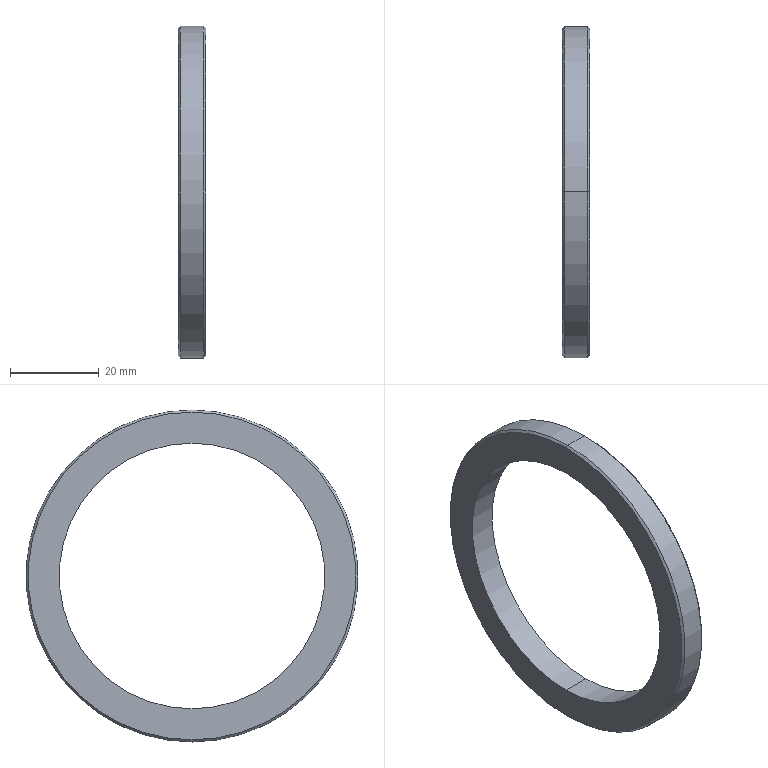Part | SolidWorks | features MBimport 1 | 1 solid | 10 faces | box 6.3 x 75 x 75 mm | volume 9961 mm3 | cone 4 | cylinder 4 | plane 2 | commonest cylinder face diameters 60 x2 75 x2
STEP:
#1=CARTESIAN_POINT('',(-37.414,0.,37.));
#2=VERTEX_POINT('',#1);
#3=CARTESIAN_POINT('',(-36.914,0.,37.5));
#4=VERTEX_POINT('',#3);
#5=CARTESIAN_POINT('',(-36.914,0.,37.5));
#6=DIRECTION('',(0.7071,0.,0.7071));
#7=VECTOR('',#6,1000.);
#8=LINE('',#5,#7);
#9=EDGE_CURVE('',#2,#4,#8,.T.);
#10=ORIENTED_EDGE('',*,*,#9,.F.);
#11=CARTESIAN_POINT('',(-37.414,0.,-37.));
#12=VERTEX_POINT('',#11);
#13=CARTESIAN_POINT('',(-37.414,0.,0.));
#14=DIRECTION('',(-1.,0.,0.));
#15=DIRECTION('',(0.,0.,1.));
#16=AXIS2_PLACEMENT_3D('',#13,#14,#15);
#17=CIRCLE('',#16,37.);
#18=EDGE_CURVE('',#12,#2,#17,.T.);
#19=ORIENTED_EDGE('',*,*,#18,.F.);
#20=CARTESIAN_POINT('',(-36.914,0.,-37.5));
#21=VERTEX_POINT('',#20);
#22=CARTESIAN_POINT('',(-36.914,0.,-37.5));
#23=DIRECTION('',(0.7071,0.,-0.7071));
#24=VECTOR('',#23,1000.);
#25=LINE('',#22,#24);
#26=EDGE_CURVE('',#12,#21,#25,.T.);
#27=ORIENTED_EDGE('',*,*,#26,.T.);
#28=CARTESIAN_POINT('',(-36.914,0.,0.));
#29=DIRECTION('',(1.,0.,0.));
#30=DIRECTION('',(0.,0.,1.));
#31=AXIS2_PLACEMENT_3D('',#28,#29,#30);
#32=CIRCLE('',#31,37.5);
#33=EDGE_CURVE('',#4,#21,#32,.T.);
#34=ORIENTED_EDGE('',*,*,#33,.F.);
#35=EDGE_LOOP('',(#10,#19,#27,#34));
#36=FACE_OUTER_BOUND('',#35,.T.);
#37=CARTESIAN_POINT('',(-36.914,0.,0.));
#38=DIRECTION('',(1.,0.,0.));
#39=DIRECTION('',(0.,0.,-1.));
#40=AXIS2_PLACEMENT_3D('',#37,#38,#39);
#41=CONICAL_SURFACE('',#40,37.5,0.7854);
#42=ADVANCED_FACE('',(#36),#41,.T.);
#43=CARTESIAN_POINT('',(-31.114,0.,-37.));
#44=VERTEX_POINT('',#43);
#45=CARTESIAN_POINT('',(-31.614,0.,-37.5));
#46=VERTEX_POINT('',#45);
#47=CARTESIAN_POINT('',(-31.114,0.,-37.));
#48=DIRECTION('',(-0.7071,0.,-0.7071));
#49=VECTOR('',#48,1000.);
#50=LINE('',#47,#49);
#51=EDGE_CURVE('',#44,#46,#50,.T.);
#52=ORIENTED_EDGE('',*,*,#51,.F.);
#53=CARTESIAN_POINT('',(-31.114,0.,37.));
#54=VERTEX_POINT('',#53);
#55=CARTESIAN_POINT('',(-31.114,0.,0.));
#56=DIRECTION('',(1.,0.,0.));
#57=DIRECTION('',(0.,0.,-1.));
#58=AXIS2_PLACEMENT_3D('',#55,#56,#57);
#59=CIRCLE('',#58,37.);
#60=EDGE_CURVE('',#54,#44,#59,.T.);
#61=ORIENTED_EDGE('',*,*,#60,.F.);
#62=CARTESIAN_POINT('',(-31.614,0.,37.5));
#63=VERTEX_POINT('',#62);
#64=CARTESIAN_POINT('',(-31.114,0.,37.));
#65=DIRECTION('',(-0.7071,0.,0.7071));
#66=VECTOR('',#65,1000.);
#67=LINE('',#64,#66);
#68=EDGE_CURVE('',#54,#63,#67,.T.);
#69=ORIENTED_EDGE('',*,*,#68,.T.);
#70=CARTESIAN_POINT('',(-31.614,0.,0.));
#71=DIRECTION('',(-1.,0.,0.));
#72=DIRECTION('',(0.,0.,-1.));
#73=AXIS2_PLACEMENT_3D('',#70,#71,#72);
#74=CIRCLE('',#73,37.5);
#75=EDGE_CURVE('',#46,#63,#74,.T.);
#76=ORIENTED_EDGE('',*,*,#75,.F.);
#77=EDGE_LOOP('',(#52,#61,#69,#76));
#78=FACE_OUTER_BOUND('',#77,.T.);
#79=CARTESIAN_POINT('',(-31.114,0.,0.));
#80=DIRECTION('',(-1.,0.,0.));
#81=DIRECTION('',(0.,0.,1.));
#82=AXIS2_PLACEMENT_3D('',#79,#80,#81);
#83=CONICAL_SURFACE('',#82,37.,0.7854);
#84=ADVANCED_FACE('',(#78),#83,.T.);
#85=CARTESIAN_POINT('',(0.,0.,37.5));
#86=DIRECTION('',(1.,0.,0.));
#87=VECTOR('',#86,1000.);
#88=LINE('',#85,#87);
#89=EDGE_CURVE('',#4,#63,#88,.T.);
#90=ORIENTED_EDGE('',*,*,#89,.F.);
#91=ORIENTED_EDGE('',*,*,#33,.T.);
#92=CARTESIAN_POINT('',(0.,0.,-37.5));
#93=DIRECTION('',(1.,0.,0.));
#94=VECTOR('',#93,1000.);
#95=LINE('',#92,#94);
#96=EDGE_CURVE('',#21,#46,#95,.T.);
#97=ORIENTED_EDGE('',*,*,#96,.T.);
#98=ORIENTED_EDGE('',*,*,#75,.T.);
#99=EDGE_LOOP('',(#90,#91,#97,#98));
#100=FACE_OUTER_BOUND('',#99,.T.);
#101=CARTESIAN_POINT('',(0.,0.,0.));
#102=DIRECTION('',(1.,0.,0.));
#103=DIRECTION('',(0.,0.,-1.));
#104=AXIS2_PLACEMENT_3D('',#101,#102,#103);
#105=CYLINDRICAL_SURFACE('',#104,37.5);
#106=ADVANCED_FACE('',(#100),#105,.T.);
#107=CARTESIAN_POINT('',(-31.114,0.,-30.));
#108=VERTEX_POINT('',#107);
#109=CARTESIAN_POINT('',(-31.114,0.,30.));
#110=VERTEX_POINT('',#109);
#111=CARTESIAN_POINT('',(-31.114,0.,0.));
#112=DIRECTION('',(1.,0.,0.));
#113=DIRECTION('',(0.,0.,-1.));
#114=AXIS2_PLACEMENT_3D('',#111,#112,#113);
#115=CIRCLE('',#114,30.);
#116=EDGE_CURVE('',#108,#110,#115,.T.);
#117=ORIENTED_EDGE('',*,*,#116,.F.);
#118=CARTESIAN_POINT('',(-31.114,0.,0.));
#119=DIRECTION('',(1.,0.,0.));
#120=DIRECTION('',(0.,0.,-1.));
#121=AXIS2_PLACEMENT_3D('',#118,#119,#120);
#122=CIRCLE('',#121,30.);
#123=EDGE_CURVE('',#110,#108,#122,.T.);
#124=ORIENTED_EDGE('',*,*,#123,.F.);
#125=EDGE_LOOP('',(#117,#124));
#126=FACE_BOUND('',#125,.T.);
#127=ORIENTED_EDGE('',*,*,#60,.T.);
#128=CARTESIAN_POINT('',(-31.114,0.,0.));
#129=DIRECTION('',(1.,0.,0.));
#130=DIRECTION('',(0.,0.,-1.));
#131=AXIS2_PLACEMENT_3D('',#128,#129,#130);
#132=CIRCLE('',#131,37.);
#133=EDGE_CURVE('',#44,#54,#132,.T.);
#134=ORIENTED_EDGE('',*,*,#133,.T.);
#135=EDGE_LOOP('',(#127,#134));
#136=FACE_OUTER_BOUND('',#135,.T.);
#137=CARTESIAN_POINT('',(-31.114,37.5,0.));
#138=DIRECTION('',(1.,0.,0.));
#139=DIRECTION('',(0.,1.,0.));
#140=AXIS2_PLACEMENT_3D('',#137,#138,#139);
#141=PLANE('',#140);
#142=ADVANCED_FACE('',(#126,#136),#141,.T.);
#143=CARTESIAN_POINT('',(-37.414,0.,30.));
#144=VERTEX_POINT('',#143);
#145=CARTESIAN_POINT('',(0.,0.,30.));
#146=DIRECTION('',(1.,0.,0.));
#147=VECTOR('',#146,1000.);
#148=LINE('',#145,#147);
#149=EDGE_CURVE('',#144,#110,#148,.T.);
#150=ORIENTED_EDGE('',*,*,#149,.F.);
#151=CARTESIAN_POINT('',(-37.414,0.,-30.));
#152=VERTEX_POINT('',#151);
#153=CARTESIAN_POINT('',(-37.414,0.,0.));
#154=DIRECTION('',(1.,0.,0.));
#155=DIRECTION('',(0.,0.,-1.));
#156=AXIS2_PLACEMENT_3D('',#153,#154,#155);
#157=CIRCLE('',#156,30.);
#158=EDGE_CURVE('',#152,#144,#157,.T.);
#159=ORIENTED_EDGE('',*,*,#158,.F.);
#160=CARTESIAN_POINT('',(0.,0.,-30.));
#161=DIRECTION('',(1.,0.,0.));
#162=VECTOR('',#161,1000.);
#163=LINE('',#160,#162);
#164=EDGE_CURVE('',#152,#108,#163,.T.);
#165=ORIENTED_EDGE('',*,*,#164,.T.);
#166=ORIENTED_EDGE('',*,*,#116,.T.);
#167=EDGE_LOOP('',(#150,#159,#165,#166));
#168=FACE_OUTER_BOUND('',#167,.T.);
#169=CARTESIAN_POINT('',(0.,0.,0.));
#170=DIRECTION('',(1.,0.,0.));
#171=DIRECTION('',(0.,0.,-1.));
#172=AXIS2_PLACEMENT_3D('',#169,#170,#171);
#173=CYLINDRICAL_SURFACE('',#172,30.);
#174=ADVANCED_FACE('',(#168),#173,.F.);
#175=ORIENTED_EDGE('',*,*,#158,.T.);
#176=CARTESIAN_POINT('',(-37.414,0.,0.));
#177=DIRECTION('',(1.,0.,0.));
#178=DIRECTION('',(0.,0.,-1.));
#179=AXIS2_PLACEMENT_3D('',#176,#177,#178);
#180=CIRCLE('',#179,30.);
#181=EDGE_CURVE('',#144,#152,#180,.T.);
#182=ORIENTED_EDGE('',*,*,#181,.T.);
#183=EDGE_LOOP('',(#175,#182));
#184=FACE_BOUND('',#183,.T.);
#185=ORIENTED_EDGE('',*,*,#18,.T.);
#186=CARTESIAN_POINT('',(-37.414,0.,0.));
#187=DIRECTION('',(-1.,0.,0.));
#188=DIRECTION('',(0.,0.,1.));
#189=AXIS2_PLACEMENT_3D('',#186,#187,#188);
#190=CIRCLE('',#189,37.);
#191=EDGE_CURVE('',#2,#12,#190,.T.);
#192=ORIENTED_EDGE('',*,*,#191,.T.);
#193=EDGE_LOOP('',(#185,#192));
#194=FACE_OUTER_BOUND('',#193,.T.);
#195=CARTESIAN_POINT('',(-37.414,37.5,0.));
#196=DIRECTION('',(-1.,0.,0.));
#197=DIRECTION('',(0.,0.,1.));
#198=AXIS2_PLACEMENT_3D('',#195,#196,#197);
#199=PLANE('',#198);
#200=ADVANCED_FACE('',(#184,#194),#199,.T.);
#201=ORIENTED_EDGE('',*,*,#181,.F.);
#202=ORIENTED_EDGE('',*,*,#149,.T.);
#203=ORIENTED_EDGE('',*,*,#123,.T.);
#204=ORIENTED_EDGE('',*,*,#164,.F.);
#205=EDGE_LOOP('',(#201,#202,#203,#204));
#206=FACE_OUTER_BOUND('',#205,.T.);
#207=CARTESIAN_POINT('',(0.,0.,0.));
#208=DIRECTION('',(1.,0.,0.));
#209=DIRECTION('',(0.,0.,-1.));
#210=AXIS2_PLACEMENT_3D('',#207,#208,#209);
#211=CYLINDRICAL_SURFACE('',#210,30.);
#212=ADVANCED_FACE('',(#206),#211,.F.);
#213=CARTESIAN_POINT('',(-36.914,0.,0.));
#214=DIRECTION('',(1.,0.,0.));
#215=DIRECTION('',(0.,0.,1.));
#216=AXIS2_PLACEMENT_3D('',#213,#214,#215);
#217=CIRCLE('',#216,37.5);
#218=EDGE_CURVE('',#21,#4,#217,.T.);
#219=ORIENTED_EDGE('',*,*,#218,.T.);
#220=ORIENTED_EDGE('',*,*,#89,.T.);
#221=CARTESIAN_POINT('',(-31.614,0.,0.));
#222=DIRECTION('',(-1.,0.,0.));
#223=DIRECTION('',(0.,0.,-1.));
#224=AXIS2_PLACEMENT_3D('',#221,#222,#223);
#225=CIRCLE('',#224,37.5);
#226=EDGE_CURVE('',#63,#46,#225,.T.);
#227=ORIENTED_EDGE('',*,*,#226,.T.);
#228=ORIENTED_EDGE('',*,*,#96,.F.);
#229=EDGE_LOOP('',(#219,#220,#227,#228));
#230=FACE_OUTER_BOUND('',#229,.T.);
#231=CARTESIAN_POINT('',(0.,0.,0.));
#232=DIRECTION('',(1.,0.,0.));
#233=DIRECTION('',(0.,0.,-1.));
#234=AXIS2_PLACEMENT_3D('',#231,#232,#233);
#235=CYLINDRICAL_SURFACE('',#234,37.5);
#236=ADVANCED_FACE('',(#230),#235,.T.);
#237=ORIENTED_EDGE('',*,*,#133,.F.);
#238=ORIENTED_EDGE('',*,*,#51,.T.);
#239=ORIENTED_EDGE('',*,*,#226,.F.);
#240=ORIENTED_EDGE('',*,*,#68,.F.);
#241=EDGE_LOOP('',(#237,#238,#239,#240));
#242=FACE_OUTER_BOUND('',#241,.T.);
#243=CARTESIAN_POINT('',(-31.114,0.,0.));
#244=DIRECTION('',(-1.,0.,0.));
#245=DIRECTION('',(0.,0.,1.));
#246=AXIS2_PLACEMENT_3D('',#243,#244,#245);
#247=CONICAL_SURFACE('',#246,37.,0.7854);
#248=ADVANCED_FACE('',(#242),#247,.T.);
#249=ORIENTED_EDGE('',*,*,#191,.F.);
#250=ORIENTED_EDGE('',*,*,#9,.T.);
#251=ORIENTED_EDGE('',*,*,#218,.F.);
#252=ORIENTED_EDGE('',*,*,#26,.F.);
#253=EDGE_LOOP('',(#249,#250,#251,#252));
#254=FACE_OUTER_BOUND('',#253,.T.);
#255=CARTESIAN_POINT('',(-36.914,0.,0.));
#256=DIRECTION('',(1.,0.,0.));
#257=DIRECTION('',(0.,0.,-1.));
#258=AXIS2_PLACEMENT_3D('',#255,#256,#257);
#259=CONICAL_SURFACE('',#258,37.5,0.7854);
#260=ADVANCED_FACE('',(#254),#259,.T.);
#261=CLOSED_SHELL('',(#42,#84,#106,#142,#174,#200,#212,#236,#248,#260));
#262=MANIFOLD_SOLID_BREP('',#261);
#263=CARTESIAN_POINT('',(0.,0.,0.));
#264=DIRECTION('',(0.,0.,1.));
#265=DIRECTION('',(1.,0.,0.));
#266=AXIS2_PLACEMENT_3D('',#263,#264,#265);
#267=(LENGTH_UNIT()NAMED_UNIT(*)SI_UNIT(.MILLI.,.METRE.));
#268=UNCERTAINTY_MEASURE_WITH_UNIT(LENGTH_MEASURE(0.00001),#267,'','');
#269=(NAMED_UNIT(*)PLANE_ANGLE_UNIT()SI_UNIT($,.RADIAN.));
#270=(NAMED_UNIT(*)SI_UNIT($,.STERADIAN.)SOLID_ANGLE_UNIT());
#271=(GEOMETRIC_REPRESENTATION_CONTEXT(3)GLOBAL_UNCERTAINTY_ASSIGNED_CONTEXT((#268))GLOBAL_UNIT_ASSIGNED_CONTEXT((#267,#269,#270))REPRESENTATION_CONTEXT('',''));
#272=ADVANCED_BREP_SHAPE_REPRESENTATION('',(#262,#266),#271);